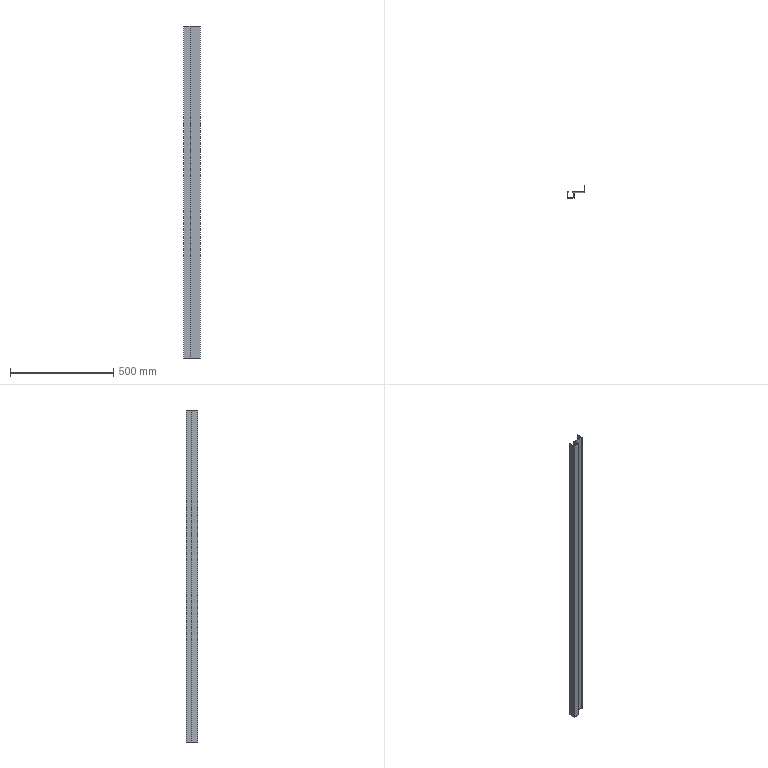Part | STEP file | Rieles_2-23 | 1 solid | 18 faces | box 81.4 x 57.7 x 1608 mm | volume 418964 mm3 | plane 18
STEP:
#1=CARTESIAN_POINT('',(10.,26.2,-551.));
#2=VERTEX_POINT('',#1);
#3=CARTESIAN_POINT('',(10.,27.7,-551.));
#4=VERTEX_POINT('',#3);
#5=CARTESIAN_POINT('',(10.,27.35,-551.));
#6=DIRECTION('',(0.,1.,0.));
#7=VECTOR('',#6,1000.);
#8=LINE('',#5,#7);
#9=EDGE_CURVE('',#2,#4,#8,.T.);
#10=ORIENTED_EDGE('',*,*,#9,.T.);
#11=CARTESIAN_POINT('',(64.2,27.7,-551.));
#12=VERTEX_POINT('',#11);
#13=CARTESIAN_POINT('',(25.,27.7,-551.));
#14=DIRECTION('',(1.,0.,0.));
#15=VECTOR('',#14,1000.);
#16=LINE('',#13,#15);
#17=EDGE_CURVE('',#4,#12,#16,.T.);
#18=ORIENTED_EDGE('',*,*,#17,.T.);
#19=CARTESIAN_POINT('',(64.2,56.2,-551.));
#20=VERTEX_POINT('',#19);
#21=CARTESIAN_POINT('',(64.2,27.35,-551.));
#22=DIRECTION('',(0.,1.,0.));
#23=VECTOR('',#22,1000.);
#24=LINE('',#21,#23);
#25=EDGE_CURVE('',#12,#20,#24,.T.);
#26=ORIENTED_EDGE('',*,*,#25,.T.);
#27=CARTESIAN_POINT('',(65.7,56.2,-551.));
#28=VERTEX_POINT('',#27);
#29=CARTESIAN_POINT('',(25.,56.2,-551.));
#30=DIRECTION('',(1.,0.,0.));
#31=VECTOR('',#30,1000.);
#32=LINE('',#29,#31);
#33=EDGE_CURVE('',#20,#28,#32,.T.);
#34=ORIENTED_EDGE('',*,*,#33,.T.);
#35=CARTESIAN_POINT('',(65.7,26.2,-551.));
#36=VERTEX_POINT('',#35);
#37=CARTESIAN_POINT('',(65.7,27.35,-551.));
#38=DIRECTION('',(0.,-1.,0.));
#39=VECTOR('',#38,1000.);
#40=LINE('',#37,#39);
#41=EDGE_CURVE('',#28,#36,#40,.T.);
#42=ORIENTED_EDGE('',*,*,#41,.T.);
#43=CARTESIAN_POINT('',(15.7,26.2,-551.));
#44=VERTEX_POINT('',#43);
#45=CARTESIAN_POINT('',(25.,26.2,-551.));
#46=DIRECTION('',(-1.,0.,0.));
#47=VECTOR('',#46,1000.);
#48=LINE('',#45,#47);
#49=EDGE_CURVE('',#36,#44,#48,.T.);
#50=ORIENTED_EDGE('',*,*,#49,.T.);
#51=CARTESIAN_POINT('',(15.7,-1.5,-551.));
#52=VERTEX_POINT('',#51);
#53=CARTESIAN_POINT('',(15.7,27.35,-551.));
#54=DIRECTION('',(0.,-1.,0.));
#55=VECTOR('',#54,1000.);
#56=LINE('',#53,#55);
#57=EDGE_CURVE('',#44,#52,#56,.T.);
#58=ORIENTED_EDGE('',*,*,#57,.T.);
#59=CARTESIAN_POINT('',(-15.7,-1.5,-551.));
#60=VERTEX_POINT('',#59);
#61=CARTESIAN_POINT('',(25.,-1.5,-551.));
#62=DIRECTION('',(-1.,0.,0.));
#63=VECTOR('',#62,1000.);
#64=LINE('',#61,#63);
#65=EDGE_CURVE('',#52,#60,#64,.T.);
#66=ORIENTED_EDGE('',*,*,#65,.T.);
#67=CARTESIAN_POINT('',(-15.7,27.7,-551.));
#68=VERTEX_POINT('',#67);
#69=CARTESIAN_POINT('',(-15.7,27.35,-551.));
#70=DIRECTION('',(0.,1.,0.));
#71=VECTOR('',#70,1000.);
#72=LINE('',#69,#71);
#73=EDGE_CURVE('',#60,#68,#72,.T.);
#74=ORIENTED_EDGE('',*,*,#73,.T.);
#75=CARTESIAN_POINT('',(-10.,27.7,-551.));
#76=VERTEX_POINT('',#75);
#77=CARTESIAN_POINT('',(25.,27.7,-551.));
#78=DIRECTION('',(1.,0.,0.));
#79=VECTOR('',#78,1000.);
#80=LINE('',#77,#79);
#81=EDGE_CURVE('',#68,#76,#80,.T.);
#82=ORIENTED_EDGE('',*,*,#81,.T.);
#83=CARTESIAN_POINT('',(-10.,26.2,-551.));
#84=VERTEX_POINT('',#83);
#85=CARTESIAN_POINT('',(-10.,27.35,-551.));
#86=DIRECTION('',(0.,-1.,0.));
#87=VECTOR('',#86,1000.);
#88=LINE('',#85,#87);
#89=EDGE_CURVE('',#76,#84,#88,.T.);
#90=ORIENTED_EDGE('',*,*,#89,.T.);
#91=CARTESIAN_POINT('',(-14.2,26.2,-551.));
#92=VERTEX_POINT('',#91);
#93=CARTESIAN_POINT('',(25.,26.2,-551.));
#94=DIRECTION('',(-1.,0.,0.));
#95=VECTOR('',#94,1000.);
#96=LINE('',#93,#95);
#97=EDGE_CURVE('',#84,#92,#96,.T.);
#98=ORIENTED_EDGE('',*,*,#97,.T.);
#99=CARTESIAN_POINT('',(-14.2,0.,-551.));
#100=VERTEX_POINT('',#99);
#101=CARTESIAN_POINT('',(-14.2,27.35,-551.));
#102=DIRECTION('',(0.,-1.,0.));
#103=VECTOR('',#102,1000.);
#104=LINE('',#101,#103);
#105=EDGE_CURVE('',#92,#100,#104,.T.);
#106=ORIENTED_EDGE('',*,*,#105,.T.);
#107=CARTESIAN_POINT('',(14.2,0.,-551.));
#108=VERTEX_POINT('',#107);
#109=CARTESIAN_POINT('',(25.,0.,-551.));
#110=DIRECTION('',(1.,0.,0.));
#111=VECTOR('',#110,1000.);
#112=LINE('',#109,#111);
#113=EDGE_CURVE('',#100,#108,#112,.T.);
#114=ORIENTED_EDGE('',*,*,#113,.T.);
#115=CARTESIAN_POINT('',(14.2,26.2,-551.));
#116=VERTEX_POINT('',#115);
#117=CARTESIAN_POINT('',(14.2,27.35,-551.));
#118=DIRECTION('',(0.,1.,0.));
#119=VECTOR('',#118,1000.);
#120=LINE('',#117,#119);
#121=EDGE_CURVE('',#108,#116,#120,.T.);
#122=ORIENTED_EDGE('',*,*,#121,.T.);
#123=CARTESIAN_POINT('',(25.,26.2,-551.));
#124=DIRECTION('',(-1.,0.,0.));
#125=VECTOR('',#124,1000.);
#126=LINE('',#123,#125);
#127=EDGE_CURVE('',#116,#2,#126,.T.);
#128=ORIENTED_EDGE('',*,*,#127,.T.);
#129=EDGE_LOOP('',(#10,#18,#26,#34,#42,#50,#58,#66,#74,#82,#90,#98,#106,#114,#122,#128));
#130=FACE_OUTER_BOUND('',#129,.T.);
#131=CARTESIAN_POINT('',(25.,27.35,-551.));
#132=DIRECTION('',(0.,0.,-1.));
#133=DIRECTION('',(0.,-1.,0.));
#134=AXIS2_PLACEMENT_3D('',#131,#132,#133);
#135=PLANE('',#134);
#136=ADVANCED_FACE('',(#130),#135,.T.);
#137=CARTESIAN_POINT('',(10.,26.2,1057.));
#138=VERTEX_POINT('',#137);
#139=CARTESIAN_POINT('',(10.,27.7,1057.));
#140=VERTEX_POINT('',#139);
#141=CARTESIAN_POINT('',(10.,26.2,1057.));
#142=DIRECTION('',(0.,1.,0.));
#143=VECTOR('',#142,1000.);
#144=LINE('',#141,#143);
#145=EDGE_CURVE('',#138,#140,#144,.T.);
#146=ORIENTED_EDGE('',*,*,#145,.F.);
#147=CARTESIAN_POINT('',(14.2,26.2,1057.));
#148=VERTEX_POINT('',#147);
#149=CARTESIAN_POINT('',(14.2,26.2,1057.));
#150=DIRECTION('',(-1.,0.,0.));
#151=VECTOR('',#150,1000.);
#152=LINE('',#149,#151);
#153=EDGE_CURVE('',#148,#138,#152,.T.);
#154=ORIENTED_EDGE('',*,*,#153,.F.);
#155=CARTESIAN_POINT('',(14.2,0.,1057.));
#156=VERTEX_POINT('',#155);
#157=CARTESIAN_POINT('',(14.2,0.,1057.));
#158=DIRECTION('',(0.,1.,0.));
#159=VECTOR('',#158,1000.);
#160=LINE('',#157,#159);
#161=EDGE_CURVE('',#156,#148,#160,.T.);
#162=ORIENTED_EDGE('',*,*,#161,.F.);
#163=CARTESIAN_POINT('',(-14.2,0.,1057.));
#164=VERTEX_POINT('',#163);
#165=CARTESIAN_POINT('',(-14.2,0.,1057.));
#166=DIRECTION('',(1.,0.,0.));
#167=VECTOR('',#166,1000.);
#168=LINE('',#165,#167);
#169=EDGE_CURVE('',#164,#156,#168,.T.);
#170=ORIENTED_EDGE('',*,*,#169,.F.);
#171=CARTESIAN_POINT('',(-14.2,26.2,1057.));
#172=VERTEX_POINT('',#171);
#173=CARTESIAN_POINT('',(-14.2,26.2,1057.));
#174=DIRECTION('',(0.,-1.,0.));
#175=VECTOR('',#174,1000.);
#176=LINE('',#173,#175);
#177=EDGE_CURVE('',#172,#164,#176,.T.);
#178=ORIENTED_EDGE('',*,*,#177,.F.);
#179=CARTESIAN_POINT('',(-10.,26.2,1057.));
#180=VERTEX_POINT('',#179);
#181=CARTESIAN_POINT('',(-10.,26.2,1057.));
#182=DIRECTION('',(-1.,0.,0.));
#183=VECTOR('',#182,1000.);
#184=LINE('',#181,#183);
#185=EDGE_CURVE('',#180,#172,#184,.T.);
#186=ORIENTED_EDGE('',*,*,#185,.F.);
#187=CARTESIAN_POINT('',(-10.,27.7,1057.));
#188=VERTEX_POINT('',#187);
#189=CARTESIAN_POINT('',(-10.,27.7,1057.));
#190=DIRECTION('',(0.,-1.,0.));
#191=VECTOR('',#190,1000.);
#192=LINE('',#189,#191);
#193=EDGE_CURVE('',#188,#180,#192,.T.);
#194=ORIENTED_EDGE('',*,*,#193,.F.);
#195=CARTESIAN_POINT('',(-15.7,27.7,1057.));
#196=VERTEX_POINT('',#195);
#197=CARTESIAN_POINT('',(-15.7,27.7,1057.));
#198=DIRECTION('',(1.,0.,0.));
#199=VECTOR('',#198,1000.);
#200=LINE('',#197,#199);
#201=EDGE_CURVE('',#196,#188,#200,.T.);
#202=ORIENTED_EDGE('',*,*,#201,.F.);
#203=CARTESIAN_POINT('',(-15.7,-1.5,1057.));
#204=VERTEX_POINT('',#203);
#205=CARTESIAN_POINT('',(-15.7,-1.5,1057.));
#206=DIRECTION('',(0.,1.,0.));
#207=VECTOR('',#206,1000.);
#208=LINE('',#205,#207);
#209=EDGE_CURVE('',#204,#196,#208,.T.);
#210=ORIENTED_EDGE('',*,*,#209,.F.);
#211=CARTESIAN_POINT('',(15.7,-1.5,1057.));
#212=VERTEX_POINT('',#211);
#213=CARTESIAN_POINT('',(15.7,-1.5,1057.));
#214=DIRECTION('',(-1.,0.,0.));
#215=VECTOR('',#214,1000.);
#216=LINE('',#213,#215);
#217=EDGE_CURVE('',#212,#204,#216,.T.);
#218=ORIENTED_EDGE('',*,*,#217,.F.);
#219=CARTESIAN_POINT('',(15.7,26.2,1057.));
#220=VERTEX_POINT('',#219);
#221=CARTESIAN_POINT('',(15.7,26.2,1057.));
#222=DIRECTION('',(0.,-1.,0.));
#223=VECTOR('',#222,1000.);
#224=LINE('',#221,#223);
#225=EDGE_CURVE('',#220,#212,#224,.T.);
#226=ORIENTED_EDGE('',*,*,#225,.F.);
#227=CARTESIAN_POINT('',(65.7,26.2,1057.));
#228=VERTEX_POINT('',#227);
#229=CARTESIAN_POINT('',(65.7,26.2,1057.));
#230=DIRECTION('',(-1.,0.,0.));
#231=VECTOR('',#230,1000.);
#232=LINE('',#229,#231);
#233=EDGE_CURVE('',#228,#220,#232,.T.);
#234=ORIENTED_EDGE('',*,*,#233,.F.);
#235=CARTESIAN_POINT('',(65.7,56.2,1057.));
#236=VERTEX_POINT('',#235);
#237=CARTESIAN_POINT('',(65.7,56.2,1057.));
#238=DIRECTION('',(0.,-1.,0.));
#239=VECTOR('',#238,1000.);
#240=LINE('',#237,#239);
#241=EDGE_CURVE('',#236,#228,#240,.T.);
#242=ORIENTED_EDGE('',*,*,#241,.F.);
#243=CARTESIAN_POINT('',(64.2,56.2,1057.));
#244=VERTEX_POINT('',#243);
#245=CARTESIAN_POINT('',(64.2,56.2,1057.));
#246=DIRECTION('',(1.,0.,0.));
#247=VECTOR('',#246,1000.);
#248=LINE('',#245,#247);
#249=EDGE_CURVE('',#244,#236,#248,.T.);
#250=ORIENTED_EDGE('',*,*,#249,.F.);
#251=CARTESIAN_POINT('',(64.2,27.7,1057.));
#252=VERTEX_POINT('',#251);
#253=CARTESIAN_POINT('',(64.2,27.7,1057.));
#254=DIRECTION('',(0.,1.,0.));
#255=VECTOR('',#254,1000.);
#256=LINE('',#253,#255);
#257=EDGE_CURVE('',#252,#244,#256,.T.);
#258=ORIENTED_EDGE('',*,*,#257,.F.);
#259=CARTESIAN_POINT('',(10.,27.7,1057.));
#260=DIRECTION('',(1.,0.,0.));
#261=VECTOR('',#260,1000.);
#262=LINE('',#259,#261);
#263=EDGE_CURVE('',#140,#252,#262,.T.);
#264=ORIENTED_EDGE('',*,*,#263,.F.);
#265=EDGE_LOOP('',(#146,#154,#162,#170,#178,#186,#194,#202,#210,#218,#226,#234,#242,#250,#258,#264));
#266=FACE_OUTER_BOUND('',#265,.T.);
#267=CARTESIAN_POINT('',(25.,27.35,1057.));
#268=DIRECTION('',(0.,0.,1.));
#269=DIRECTION('',(1.,0.,0.));
#270=AXIS2_PLACEMENT_3D('',#267,#268,#269);
#271=PLANE('',#270);
#272=ADVANCED_FACE('',(#266),#271,.T.);
#273=ORIENTED_EDGE('',*,*,#145,.T.);
#274=CARTESIAN_POINT('',(10.,27.7,407.));
#275=DIRECTION('',(0.,0.,-1.));
#276=VECTOR('',#275,1000.);
#277=LINE('',#274,#276);
#278=EDGE_CURVE('',#140,#4,#277,.T.);
#279=ORIENTED_EDGE('',*,*,#278,.T.);
#280=ORIENTED_EDGE('',*,*,#9,.F.);
#281=CARTESIAN_POINT('',(10.,26.2,407.));
#282=DIRECTION('',(0.,0.,-1.));
#283=VECTOR('',#282,1000.);
#284=LINE('',#281,#283);
#285=EDGE_CURVE('',#138,#2,#284,.T.);
#286=ORIENTED_EDGE('',*,*,#285,.F.);
#287=EDGE_LOOP('',(#273,#279,#280,#286));
#288=FACE_OUTER_BOUND('',#287,.T.);
#289=CARTESIAN_POINT('',(10.,26.2,407.));
#290=DIRECTION('',(-1.,0.,0.));
#291=DIRECTION('',(0.,0.,1.));
#292=AXIS2_PLACEMENT_3D('',#289,#290,#291);
#293=PLANE('',#292);
#294=ADVANCED_FACE('',(#288),#293,.T.);
#295=ORIENTED_EDGE('',*,*,#263,.T.);
#296=CARTESIAN_POINT('',(64.2,27.7,407.));
#297=DIRECTION('',(0.,0.,-1.));
#298=VECTOR('',#297,1000.);
#299=LINE('',#296,#298);
#300=EDGE_CURVE('',#252,#12,#299,.T.);
#301=ORIENTED_EDGE('',*,*,#300,.T.);
#302=ORIENTED_EDGE('',*,*,#17,.F.);
#303=ORIENTED_EDGE('',*,*,#278,.F.);
#304=EDGE_LOOP('',(#295,#301,#302,#303));
#305=FACE_OUTER_BOUND('',#304,.T.);
#306=CARTESIAN_POINT('',(10.,27.7,407.));
#307=DIRECTION('',(0.,1.,0.));
#308=DIRECTION('',(1.,0.,0.));
#309=AXIS2_PLACEMENT_3D('',#306,#307,#308);
#310=PLANE('',#309);
#311=ADVANCED_FACE('',(#305),#310,.T.);
#312=ORIENTED_EDGE('',*,*,#257,.T.);
#313=CARTESIAN_POINT('',(64.2,56.2,407.));
#314=DIRECTION('',(0.,0.,-1.));
#315=VECTOR('',#314,1000.);
#316=LINE('',#313,#315);
#317=EDGE_CURVE('',#244,#20,#316,.T.);
#318=ORIENTED_EDGE('',*,*,#317,.T.);
#319=ORIENTED_EDGE('',*,*,#25,.F.);
#320=ORIENTED_EDGE('',*,*,#300,.F.);
#321=EDGE_LOOP('',(#312,#318,#319,#320));
#322=FACE_OUTER_BOUND('',#321,.T.);
#323=CARTESIAN_POINT('',(64.2,27.7,407.));
#324=DIRECTION('',(-1.,0.,0.));
#325=DIRECTION('',(0.,0.,1.));
#326=AXIS2_PLACEMENT_3D('',#323,#324,#325);
#327=PLANE('',#326);
#328=ADVANCED_FACE('',(#322),#327,.T.);
#329=ORIENTED_EDGE('',*,*,#249,.T.);
#330=CARTESIAN_POINT('',(65.7,56.2,407.));
#331=DIRECTION('',(0.,0.,-1.));
#332=VECTOR('',#331,1000.);
#333=LINE('',#330,#332);
#334=EDGE_CURVE('',#236,#28,#333,.T.);
#335=ORIENTED_EDGE('',*,*,#334,.T.);
#336=ORIENTED_EDGE('',*,*,#33,.F.);
#337=ORIENTED_EDGE('',*,*,#317,.F.);
#338=EDGE_LOOP('',(#329,#335,#336,#337));
#339=FACE_OUTER_BOUND('',#338,.T.);
#340=CARTESIAN_POINT('',(64.2,56.2,407.));
#341=DIRECTION('',(0.,1.,0.));
#342=DIRECTION('',(1.,0.,0.));
#343=AXIS2_PLACEMENT_3D('',#340,#341,#342);
#344=PLANE('',#343);
#345=ADVANCED_FACE('',(#339),#344,.T.);
#346=ORIENTED_EDGE('',*,*,#241,.T.);
#347=CARTESIAN_POINT('',(65.7,26.2,407.));
#348=DIRECTION('',(0.,0.,-1.));
#349=VECTOR('',#348,1000.);
#350=LINE('',#347,#349);
#351=EDGE_CURVE('',#228,#36,#350,.T.);
#352=ORIENTED_EDGE('',*,*,#351,.T.);
#353=ORIENTED_EDGE('',*,*,#41,.F.);
#354=ORIENTED_EDGE('',*,*,#334,.F.);
#355=EDGE_LOOP('',(#346,#352,#353,#354));
#356=FACE_OUTER_BOUND('',#355,.T.);
#357=CARTESIAN_POINT('',(65.7,56.2,407.));
#358=DIRECTION('',(1.,0.,0.));
#359=DIRECTION('',(0.,-1.,0.));
#360=AXIS2_PLACEMENT_3D('',#357,#358,#359);
#361=PLANE('',#360);
#362=ADVANCED_FACE('',(#356),#361,.T.);
#363=ORIENTED_EDGE('',*,*,#233,.T.);
#364=CARTESIAN_POINT('',(15.7,26.2,407.));
#365=DIRECTION('',(0.,0.,-1.));
#366=VECTOR('',#365,1000.);
#367=LINE('',#364,#366);
#368=EDGE_CURVE('',#220,#44,#367,.T.);
#369=ORIENTED_EDGE('',*,*,#368,.T.);
#370=ORIENTED_EDGE('',*,*,#49,.F.);
#371=ORIENTED_EDGE('',*,*,#351,.F.);
#372=EDGE_LOOP('',(#363,#369,#370,#371));
#373=FACE_OUTER_BOUND('',#372,.T.);
#374=CARTESIAN_POINT('',(65.7,26.2,407.));
#375=DIRECTION('',(0.,-1.,0.));
#376=DIRECTION('',(0.,0.,-1.));
#377=AXIS2_PLACEMENT_3D('',#374,#375,#376);
#378=PLANE('',#377);
#379=ADVANCED_FACE('',(#373),#378,.T.);
#380=ORIENTED_EDGE('',*,*,#225,.T.);
#381=CARTESIAN_POINT('',(15.7,-1.5,407.));
#382=DIRECTION('',(0.,0.,-1.));
#383=VECTOR('',#382,1000.);
#384=LINE('',#381,#383);
#385=EDGE_CURVE('',#212,#52,#384,.T.);
#386=ORIENTED_EDGE('',*,*,#385,.T.);
#387=ORIENTED_EDGE('',*,*,#57,.F.);
#388=ORIENTED_EDGE('',*,*,#368,.F.);
#389=EDGE_LOOP('',(#380,#386,#387,#388));
#390=FACE_OUTER_BOUND('',#389,.T.);
#391=CARTESIAN_POINT('',(15.7,26.2,407.));
#392=DIRECTION('',(1.,0.,0.));
#393=DIRECTION('',(0.,1.,0.));
#394=AXIS2_PLACEMENT_3D('',#391,#392,#393);
#395=PLANE('',#394);
#396=ADVANCED_FACE('',(#390),#395,.T.);
#397=ORIENTED_EDGE('',*,*,#217,.T.);
#398=CARTESIAN_POINT('',(-15.7,-1.5,407.));
#399=DIRECTION('',(0.,0.,-1.));
#400=VECTOR('',#399,1000.);
#401=LINE('',#398,#400);
#402=EDGE_CURVE('',#204,#60,#401,.T.);
#403=ORIENTED_EDGE('',*,*,#402,.T.);
#404=ORIENTED_EDGE('',*,*,#65,.F.);
#405=ORIENTED_EDGE('',*,*,#385,.F.);
#406=EDGE_LOOP('',(#397,#403,#404,#405));
#407=FACE_OUTER_BOUND('',#406,.T.);
#408=CARTESIAN_POINT('',(15.7,-1.5,407.));
#409=DIRECTION('',(0.,-1.,0.));
#410=DIRECTION('',(0.,0.,-1.));
#411=AXIS2_PLACEMENT_3D('',#408,#409,#410);
#412=PLANE('',#411);
#413=ADVANCED_FACE('',(#407),#412,.T.);
#414=ORIENTED_EDGE('',*,*,#209,.T.);
#415=CARTESIAN_POINT('',(-15.7,27.7,407.));
#416=DIRECTION('',(0.,0.,-1.));
#417=VECTOR('',#416,1000.);
#418=LINE('',#415,#417);
#419=EDGE_CURVE('',#196,#68,#418,.T.);
#420=ORIENTED_EDGE('',*,*,#419,.T.);
#421=ORIENTED_EDGE('',*,*,#73,.F.);
#422=ORIENTED_EDGE('',*,*,#402,.F.);
#423=EDGE_LOOP('',(#414,#420,#421,#422));
#424=FACE_OUTER_BOUND('',#423,.T.);
#425=CARTESIAN_POINT('',(-15.7,-1.5,407.));
#426=DIRECTION('',(-1.,0.,0.));
#427=DIRECTION('',(0.,0.,1.));
#428=AXIS2_PLACEMENT_3D('',#425,#426,#427);
#429=PLANE('',#428);
#430=ADVANCED_FACE('',(#424),#429,.T.);
#431=ORIENTED_EDGE('',*,*,#201,.T.);
#432=CARTESIAN_POINT('',(-10.,27.7,407.));
#433=DIRECTION('',(0.,0.,-1.));
#434=VECTOR('',#433,1000.);
#435=LINE('',#432,#434);
#436=EDGE_CURVE('',#188,#76,#435,.T.);
#437=ORIENTED_EDGE('',*,*,#436,.T.);
#438=ORIENTED_EDGE('',*,*,#81,.F.);
#439=ORIENTED_EDGE('',*,*,#419,.F.);
#440=EDGE_LOOP('',(#431,#437,#438,#439));
#441=FACE_OUTER_BOUND('',#440,.T.);
#442=CARTESIAN_POINT('',(-15.7,27.7,407.));
#443=DIRECTION('',(0.,1.,0.));
#444=DIRECTION('',(1.,0.,0.));
#445=AXIS2_PLACEMENT_3D('',#442,#443,#444);
#446=PLANE('',#445);
#447=ADVANCED_FACE('',(#441),#446,.T.);
#448=ORIENTED_EDGE('',*,*,#193,.T.);
#449=CARTESIAN_POINT('',(-10.,26.2,407.));
#450=DIRECTION('',(0.,0.,-1.));
#451=VECTOR('',#450,1000.);
#452=LINE('',#449,#451);
#453=EDGE_CURVE('',#180,#84,#452,.T.);
#454=ORIENTED_EDGE('',*,*,#453,.T.);
#455=ORIENTED_EDGE('',*,*,#89,.F.);
#456=ORIENTED_EDGE('',*,*,#436,.F.);
#457=EDGE_LOOP('',(#448,#454,#455,#456));
#458=FACE_OUTER_BOUND('',#457,.T.);
#459=CARTESIAN_POINT('',(-10.,27.7,407.));
#460=DIRECTION('',(1.,0.,0.));
#461=DIRECTION('',(0.,1.,0.));
#462=AXIS2_PLACEMENT_3D('',#459,#460,#461);
#463=PLANE('',#462);
#464=ADVANCED_FACE('',(#458),#463,.T.);
#465=ORIENTED_EDGE('',*,*,#185,.T.);
#466=CARTESIAN_POINT('',(-14.2,26.2,407.));
#467=DIRECTION('',(0.,0.,-1.));
#468=VECTOR('',#467,1000.);
#469=LINE('',#466,#468);
#470=EDGE_CURVE('',#172,#92,#469,.T.);
#471=ORIENTED_EDGE('',*,*,#470,.T.);
#472=ORIENTED_EDGE('',*,*,#97,.F.);
#473=ORIENTED_EDGE('',*,*,#453,.F.);
#474=EDGE_LOOP('',(#465,#471,#472,#473));
#475=FACE_OUTER_BOUND('',#474,.T.);
#476=CARTESIAN_POINT('',(-10.,26.2,407.));
#477=DIRECTION('',(0.,-1.,0.));
#478=DIRECTION('',(0.,0.,-1.));
#479=AXIS2_PLACEMENT_3D('',#476,#477,#478);
#480=PLANE('',#479);
#481=ADVANCED_FACE('',(#475),#480,.T.);
#482=ORIENTED_EDGE('',*,*,#177,.T.);
#483=CARTESIAN_POINT('',(-14.2,0.,407.));
#484=DIRECTION('',(0.,0.,-1.));
#485=VECTOR('',#484,1000.);
#486=LINE('',#483,#485);
#487=EDGE_CURVE('',#164,#100,#486,.T.);
#488=ORIENTED_EDGE('',*,*,#487,.T.);
#489=ORIENTED_EDGE('',*,*,#105,.F.);
#490=ORIENTED_EDGE('',*,*,#470,.F.);
#491=EDGE_LOOP('',(#482,#488,#489,#490));
#492=FACE_OUTER_BOUND('',#491,.T.);
#493=CARTESIAN_POINT('',(-14.2,26.2,407.));
#494=DIRECTION('',(1.,0.,0.));
#495=DIRECTION('',(0.,1.,0.));
#496=AXIS2_PLACEMENT_3D('',#493,#494,#495);
#497=PLANE('',#496);
#498=ADVANCED_FACE('',(#492),#497,.T.);
#499=ORIENTED_EDGE('',*,*,#169,.T.);
#500=CARTESIAN_POINT('',(14.2,0.,407.));
#501=DIRECTION('',(0.,0.,-1.));
#502=VECTOR('',#501,1000.);
#503=LINE('',#500,#502);
#504=EDGE_CURVE('',#156,#108,#503,.T.);
#505=ORIENTED_EDGE('',*,*,#504,.T.);
#506=ORIENTED_EDGE('',*,*,#113,.F.);
#507=ORIENTED_EDGE('',*,*,#487,.F.);
#508=EDGE_LOOP('',(#499,#505,#506,#507));
#509=FACE_OUTER_BOUND('',#508,.T.);
#510=CARTESIAN_POINT('',(-14.2,0.,407.));
#511=DIRECTION('',(0.,1.,0.));
#512=DIRECTION('',(1.,0.,0.));
#513=AXIS2_PLACEMENT_3D('',#510,#511,#512);
#514=PLANE('',#513);
#515=ADVANCED_FACE('',(#509),#514,.T.);
#516=ORIENTED_EDGE('',*,*,#161,.T.);
#517=CARTESIAN_POINT('',(14.2,26.2,407.));
#518=DIRECTION('',(0.,0.,-1.));
#519=VECTOR('',#518,1000.);
#520=LINE('',#517,#519);
#521=EDGE_CURVE('',#148,#116,#520,.T.);
#522=ORIENTED_EDGE('',*,*,#521,.T.);
#523=ORIENTED_EDGE('',*,*,#121,.F.);
#524=ORIENTED_EDGE('',*,*,#504,.F.);
#525=EDGE_LOOP('',(#516,#522,#523,#524));
#526=FACE_OUTER_BOUND('',#525,.T.);
#527=CARTESIAN_POINT('',(14.2,0.,407.));
#528=DIRECTION('',(-1.,0.,0.));
#529=DIRECTION('',(0.,0.,1.));
#530=AXIS2_PLACEMENT_3D('',#527,#528,#529);
#531=PLANE('',#530);
#532=ADVANCED_FACE('',(#526),#531,.T.);
#533=ORIENTED_EDGE('',*,*,#153,.T.);
#534=ORIENTED_EDGE('',*,*,#285,.T.);
#535=ORIENTED_EDGE('',*,*,#127,.F.);
#536=ORIENTED_EDGE('',*,*,#521,.F.);
#537=EDGE_LOOP('',(#533,#534,#535,#536));
#538=FACE_OUTER_BOUND('',#537,.T.);
#539=CARTESIAN_POINT('',(14.2,26.2,407.));
#540=DIRECTION('',(0.,-1.,0.));
#541=DIRECTION('',(-1.,0.,0.));
#542=AXIS2_PLACEMENT_3D('',#539,#540,#541);
#543=PLANE('',#542);
#544=ADVANCED_FACE('',(#538),#543,.T.);
#545=CLOSED_SHELL('',(#136,#272,#294,#311,#328,#345,#362,#379,#396,#413,#430,#447,#464,#481,#498,#515,#532,#544));
#546=MANIFOLD_SOLID_BREP('',#545);
#547=CARTESIAN_POINT('',(0.,0.,0.));
#548=DIRECTION('',(0.,0.,1.));
#549=DIRECTION('',(1.,0.,0.));
#550=AXIS2_PLACEMENT_3D('',#547,#548,#549);
#551=(LENGTH_UNIT()NAMED_UNIT(*)SI_UNIT(.MILLI.,.METRE.));
#552=UNCERTAINTY_MEASURE_WITH_UNIT(LENGTH_MEASURE(0.00001),#551,'','');
#553=(NAMED_UNIT(*)PLANE_ANGLE_UNIT()SI_UNIT($,.RADIAN.));
#554=(NAMED_UNIT(*)SI_UNIT($,.STERADIAN.)SOLID_ANGLE_UNIT());
#555=(GEOMETRIC_REPRESENTATION_CONTEXT(3)GLOBAL_UNCERTAINTY_ASSIGNED_CONTEXT((#552))GLOBAL_UNIT_ASSIGNED_CONTEXT((#551,#553,#554))REPRESENTATION_CONTEXT('',''));
#556=ADVANCED_BREP_SHAPE_REPRESENTATION('',(#546,#550),#555);